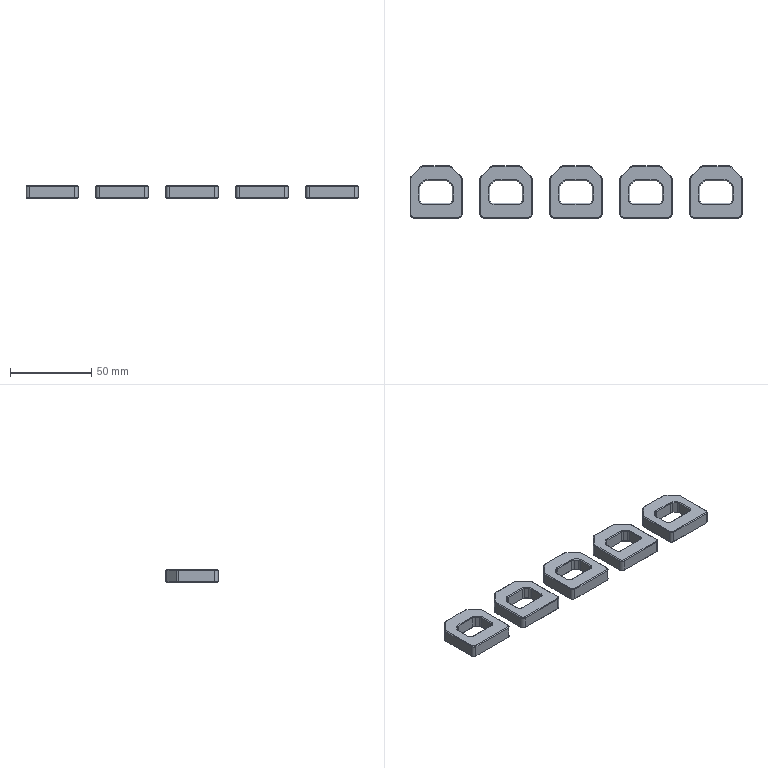NC program | NX | posted with a generic post | part box 204 x 32 x 8 mm
Whole program:
N10 G17 G21 G94 G90
(FLOOR_WALL_COPY , TOOL : D80)
N12 T19 M6
N14 G54
N16 G17 G0 G90 X147. Y0. S6500 M3
N18 G43 Z30. H19
N20 Z4.5
N22 G94 G1 Z1.5 F1500.
N24 X142.
N26 X-142.
N28 X-147.
N30 Z4.5
N32 G0 Z30.
N34 X147.
N36 Z4.
N38 G1 Z1.
N40 X142.
N42 X-142.
N44 X-147.
N46 Z4.
N48 G0 Z30.
N50 X147.
N52 Z3.5
N54 G1 Z0.5
N56 X142.
N58 X-142.
N60 X-147.
N62 Z3.5
N64 G0 Z30.
N66 X147.
N68 Z3.
N70 G1 Z0.
N72 X142.
N74 X-142.
N76 X-147.
N78 Z3.
N80 G0 Z30.
N82 M5
(PLANAR_MILL_COPY_COPY_COPY_COPY_COPY , TOOL : D6A45)
N84 T01 M6
N86 G54
N88 G17 G0 G90 X86.866 Y5.5 S9500 M3
N90 G43 Z30. H1
N92 Z0.
N94 G94 G1 Z-1.5 F1250.
N96 G3 X86. Y6. R1.
N98 G1 X78.
N100 G3 X77. Y5. R1.
N102 G1 Y-3.172
N104 G3 X77.293 Y-3.879 R1.
N106 G1 X79.121 Y-5.707
N108 G3 X79.828 Y-6. R1.
N110 G1 X92.172
N112 G3 X92.879 Y-5.707 R1.
N114 G1 X94.707 Y-3.879
N116 G3 X95. Y-3.172 R1.
N118 G1 Y5.
N120 G3 X94. Y6. R1.
N122 G1 X86.
N124 G3 X85.134 Y5.5 R1.
N126 G1 Z0.
N128 G0 Z30.
N130 Y17.5
N132 Z0.
N134 G1 Z-1.5
N136 G3 X86. Y17. R1.
N138 G1 X100.
N140 G2 X103. Y14. R3.
N142 G1 Y-8.172
N144 G2 X102.121 Y-10.293 R3.
N146 G1 X96.293 Y-16.121
N148 G2 X94.172 Y-17. R3.
N150 G1 X77.828
N152 G2 X75.707 Y-16.121 R3.
N154 G1 X69.879 Y-10.293
N156 G2 X69. Y-8.172 R3.
N158 G1 Y14.
N160 G2 X72. Y17. R3.
N162 G1 X86.
N164 G3 X86.866 Y17.5 R1.
N166 G1 Z0.
N168 G0 Z30.
N170 X42.134
N172 Z0.
N174 G1 Z-1.5
N176 G3 X43. Y17. R1.
N178 G1 X57.
N180 G2 X60. Y14. R3.
N182 G1 Y-8.172
N184 G2 X59.121 Y-10.293 R3.
N186 G1 X53.293 Y-16.121
N188 G2 X51.172 Y-17. R3.
N190 G1 X34.828
N192 G2 X32.707 Y-16.121 R3.
N194 G1 X26.879 Y-10.293
N196 G2 X26. Y-8.172 R3.
N198 G1 Y14.
N200 G2 X29. Y17. R3.
N202 G1 X43.
N204 G3 X43.866 Y17.5 R1.
N206 G1 Z0.
N208 G0 Z30.
N210 Y5.5
N212 Z0.
N214 G1 Z-1.5
N216 G3 X43. Y6. R1.
N218 G1 X35.
N220 G3 X34. Y5. R1.
N222 G1 Y-3.172
N224 G3 X34.293 Y-3.879 R1.
N226 G1 X36.121 Y-5.707
N228 G3 X36.828 Y-6. R1.
N230 G1 X49.172
N232 G3 X49.879 Y-5.707 R1.
N234 G1 X51.707 Y-3.879
N236 G3 X52. Y-3.172 R1.
N238 G1 Y5.
N240 G3 X51. Y6. R1.
N242 G1 X43.
N244 G3 X42.134 Y5.5 R1.
N246 G1 Z0.
N248 G0 Z30.
N250 X0.866
N252 Z0.
N254 G1 Z-1.5
N256 G3 X0. Y6. R1.
N258 G1 X-8.
N260 G3 X-9. Y5. R1.
N262 G1 Y-3.172
N264 G3 X-8.707 Y-3.879 R1.
N266 G1 X-6.879 Y-5.707
N268 G3 X-6.172 Y-6. R1.
N270 G1 X6.172
N272 G3 X6.879 Y-5.707 R1.
N274 G1 X8.707 Y-3.879
N276 G3 X9. Y-3.172 R1.
N278 G1 Y5.
N280 G3 X8. Y6. R1.
N282 G1 X0.
N284 G3 X-0.866 Y5.5 R1.
N286 G1 Z0.
N288 G0 Z30.
N290 Y17.5
N292 Z0.
N294 G1 Z-1.5
N296 G3 X0. Y17. R1.
N298 G1 X14.
N300 G2 X17. Y14. R3.
N302 G1 Y-8.172
N304 G2 X16.121 Y-10.293 R3.
N306 G1 X10.293 Y-16.121
N308 G2 X8.172 Y-17. R3.
N310 G1 X-8.172
N312 G2 X-10.293 Y-16.121 R3.
N314 G1 X-16.121 Y-10.293
N316 G2 X-17. Y-8.172 R3.
N318 G1 Y14.
N320 G2 X-14. Y17. R3.
N322 G1 X0.
N324 G3 X0.866 Y17.5 R1.
N326 G1 Z0.
N328 G0 Z30.
N330 X-43.866
N332 Z0.
N334 G1 Z-1.5
N336 G3 X-43. Y17. R1.
N338 G1 X-29.
N340 G2 X-26. Y14. R3.
N342 G1 Y-8.172
N344 G2 X-26.879 Y-10.293 R3.
N346 G1 X-32.707 Y-16.121
N348 G2 X-34.828 Y-17. R3.
N350 G1 X-51.172
N352 G2 X-53.293 Y-16.121 R3.
N354 G1 X-59.121 Y-10.293
N356 G2 X-60. Y-8.172 R3.
N358 G1 Y14.
N360 G2 X-57. Y17. R3.
N362 G1 X-43.
N364 G3 X-42.134 Y17.5 R1.
N366 G1 Z0.
N368 G0 Z30.
N370 Y5.5
N372 Z0.
N374 G1 Z-1.5
N376 G3 X-43. Y6. R1.
N378 G1 X-51.
N380 G3 X-52. Y5. R1.
N382 G1 Y-3.172
N384 G3 X-51.707 Y-3.879 R1.
N386 G1 X-49.879 Y-5.707
N388 G3 X-49.172 Y-6. R1.
N390 G1 X-36.828
N392 G3 X-36.121 Y-5.707 R1.
N394 G1 X-34.293 Y-3.879
N396 G3 X-34. Y-3.172 R1.
N398 G1 Y5.
N400 G3 X-35. Y6. R1.
N402 G1 X-43.
N404 G3 X-43.866 Y5.5 R1.
N406 G1 Z0.
N408 G0 Z30.
N410 X-85.134
N412 Z0.
N414 G1 Z-1.5
N416 G3 X-86. Y6. R1.
N418 G1 X-94.
N420 G3 X-95. Y5. R1.
N422 G1 Y-3.172
N424 G3 X-94.707 Y-3.879 R1.
N426 G1 X-92.879 Y-5.707
N428 G3 X-92.172 Y-6. R1.
N430 G1 X-79.828
N432 G3 X-79.121 Y-5.707 R1.
N434 G1 X-77.293 Y-3.879
N436 G3 X-77. Y-3.172 R1.
N438 G1 Y5.
N440 G3 X-78. Y6. R1.
N442 G1 X-86.
N444 G3 X-86.866 Y5.5 R1.
N446 G1 Z0.
N448 G0 Z30.
N450 Y17.5
N452 Z0.
N454 G1 Z-1.5
N456 G3 X-86. Y17. R1.
N458 G1 X-72.
N460 G2 X-69. Y14. R3.
N462 G1 Y-8.172
N464 G2 X-69.879 Y-10.293 R3.
N466 G1 X-75.707 Y-16.121
N468 G2 X-77.828 Y-17. R3.
N470 G1 X-94.172
N472 G2 X-96.293 Y-16.121 R3.
N474 G1 X-102.121 Y-10.293
N476 G2 X-103. Y-8.172 R3.
N478 G1 Y14.
N480 G2 X-100. Y17. R3.
N482 G1 X-86.
N484 G3 X-85.134 Y17.5 R1.
N486 G1 Z0.
N488 G0 Z30.
N490 M5
N492 M2